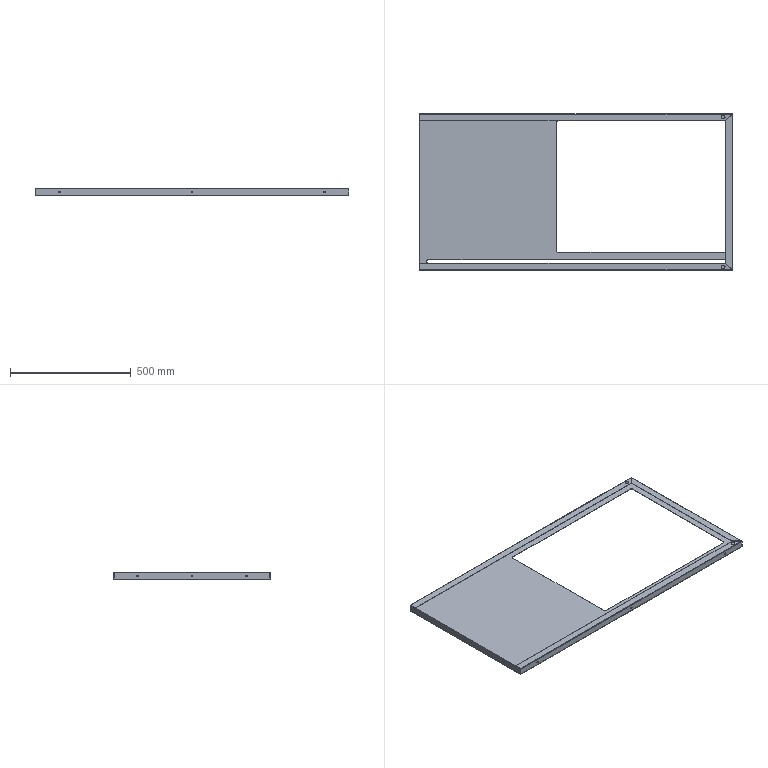Part | STEP file | Outer sheet metal | 1 solid | 108 faces | box 1300 x 650 x 30 mm | volume 960013 mm3 | cylinder 52 | plane 44 | spline 12 | commonest cylinder face diameters 7 x26 10 x8 2 x7 5 x7 15 x4